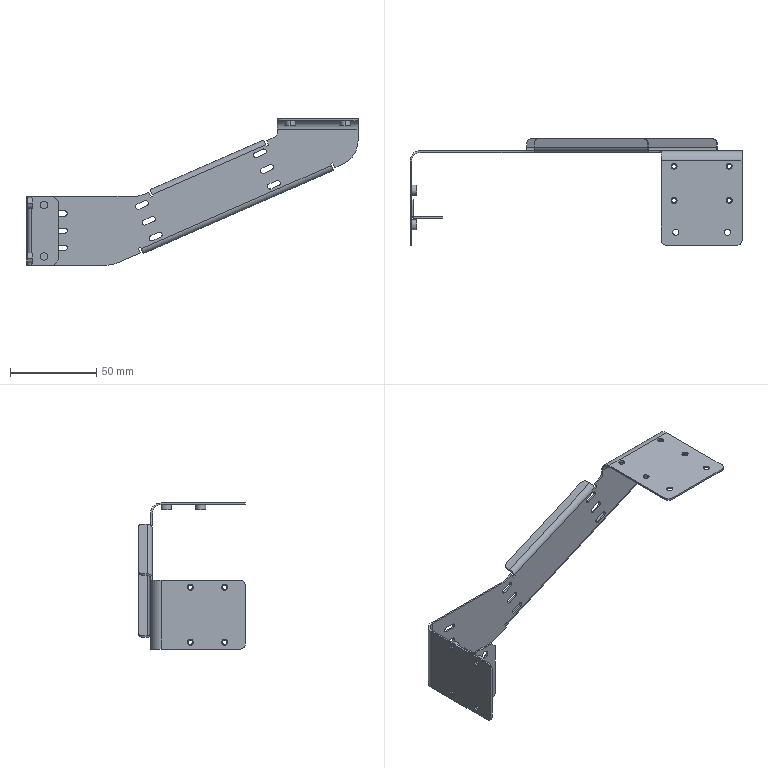Part | SolidWorks | features BaseBody 2 | 2 solids | 182 faces | box 193 x 62 x 85 mm | volume 13858 mm3 | cylinder 102 | plane 80 | commonest cylinder face diameters 6 x27 3 x24 3.5 x20 2.5 x16 4.5 x4 4 x3